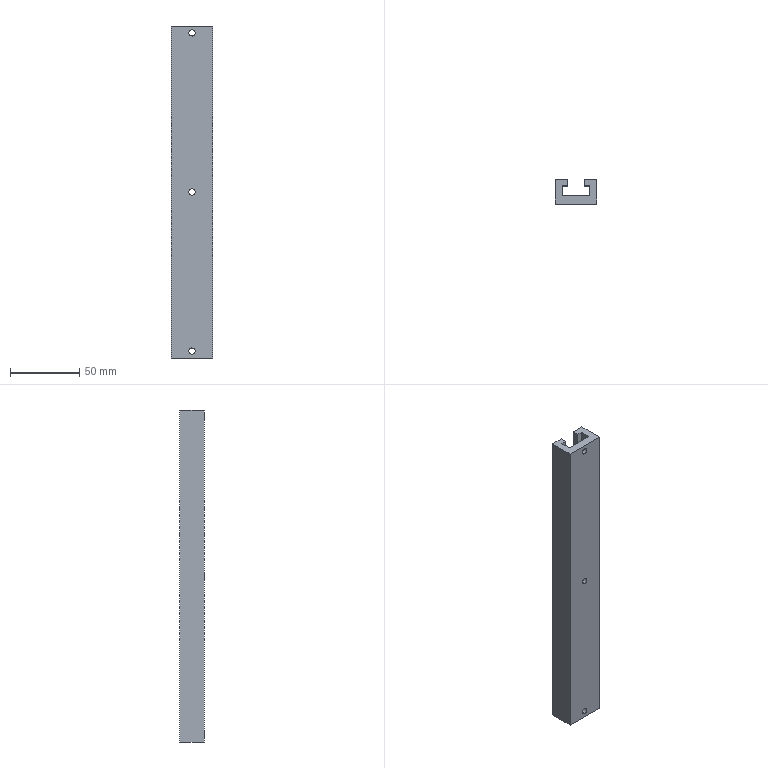Part | NX | features BREP 1 | 1 solid | 26 faces | box 30 x 18 x 240 mm | volume 80211 mm3 | plane 14 | cone 6 | cylinder 6 | commonest cylinder face diameters 4.5 x6
STEP:
#1=CARTESIAN_POINT('',(0.,6.,110.5));
#2=VERTEX_POINT('',#1);
#3=CARTESIAN_POINT('',(0.,3.75,112.75));
#4=VERTEX_POINT('',#3);
#5=CARTESIAN_POINT('',(0.,6.,110.5));
#6=DIRECTION('',(0.,0.7071,-0.7071));
#7=VECTOR('',#6,1000.);
#8=LINE('',#5,#7);
#9=EDGE_CURVE('',#2,#4,#8,.F.);
#10=ORIENTED_EDGE('',*,*,#9,.T.);
#11=CARTESIAN_POINT('',(0.,3.75,117.25));
#12=VERTEX_POINT('',#11);
#13=CARTESIAN_POINT('',(0.,3.75,115.));
#14=DIRECTION('',(0.,1.,0.));
#15=DIRECTION('',(0.,0.,1.));
#16=AXIS2_PLACEMENT_3D('',#13,#14,#15);
#17=CIRCLE('',#16,2.25);
#18=EDGE_CURVE('',#12,#4,#17,.T.);
#19=ORIENTED_EDGE('',*,*,#18,.F.);
#20=CARTESIAN_POINT('',(0.,6.,119.5));
#21=VERTEX_POINT('',#20);
#22=CARTESIAN_POINT('',(0.,6.,119.5));
#23=DIRECTION('',(0.,0.7071,0.7071));
#24=VECTOR('',#23,1000.);
#25=LINE('',#22,#24);
#26=EDGE_CURVE('',#21,#12,#25,.F.);
#27=ORIENTED_EDGE('',*,*,#26,.F.);
#28=CARTESIAN_POINT('',(0.,6.,115.));
#29=DIRECTION('',(0.,1.,0.));
#30=DIRECTION('',(0.,0.,1.));
#31=AXIS2_PLACEMENT_3D('',#28,#29,#30);
#32=CIRCLE('',#31,4.5);
#33=EDGE_CURVE('',#21,#2,#32,.T.);
#34=ORIENTED_EDGE('',*,*,#33,.T.);
#35=EDGE_LOOP('',(#10,#19,#27,#34));
#36=FACE_BOUND('',#35,.T.);
#37=CARTESIAN_POINT('',(0.,6.,115.));
#38=DIRECTION('',(0.,1.,0.));
#39=DIRECTION('',(0.,0.,1.));
#40=AXIS2_PLACEMENT_3D('',#37,#38,#39);
#41=CONICAL_SURFACE('',#40,4.5,0.7854);
#42=ADVANCED_FACE('',(#36),#41,.F.);
#43=CARTESIAN_POINT('',(0.,0.,112.75));
#44=VERTEX_POINT('',#43);
#45=CARTESIAN_POINT('',(0.,6.,112.75));
#46=DIRECTION('',(0.,1.,0.));
#47=VECTOR('',#46,1000.);
#48=LINE('',#45,#47);
#49=EDGE_CURVE('',#4,#44,#48,.F.);
#50=ORIENTED_EDGE('',*,*,#49,.T.);
#51=CARTESIAN_POINT('',(0.,0.,117.25));
#52=VERTEX_POINT('',#51);
#53=CARTESIAN_POINT('',(0.,0.,115.));
#54=DIRECTION('',(0.,1.,0.));
#55=DIRECTION('',(0.,0.,1.));
#56=AXIS2_PLACEMENT_3D('',#53,#54,#55);
#57=CIRCLE('',#56,2.25);
#58=EDGE_CURVE('',#52,#44,#57,.T.);
#59=ORIENTED_EDGE('',*,*,#58,.F.);
#60=CARTESIAN_POINT('',(0.,6.,117.25));
#61=DIRECTION('',(0.,1.,0.));
#62=VECTOR('',#61,1000.);
#63=LINE('',#60,#62);
#64=EDGE_CURVE('',#12,#52,#63,.F.);
#65=ORIENTED_EDGE('',*,*,#64,.F.);
#66=ORIENTED_EDGE('',*,*,#18,.T.);
#67=EDGE_LOOP('',(#50,#59,#65,#66));
#68=FACE_BOUND('',#67,.T.);
#69=CARTESIAN_POINT('',(0.,6.,115.));
#70=DIRECTION('',(0.,1.,0.));
#71=DIRECTION('',(0.,0.,1.));
#72=AXIS2_PLACEMENT_3D('',#69,#70,#71);
#73=CYLINDRICAL_SURFACE('',#72,2.25);
#74=ADVANCED_FACE('',(#68),#73,.F.);
#75=CARTESIAN_POINT('',(0.,6.,-4.5));
#76=VERTEX_POINT('',#75);
#77=CARTESIAN_POINT('',(0.,3.75,-2.25));
#78=VERTEX_POINT('',#77);
#79=CARTESIAN_POINT('',(0.,6.,-4.5));
#80=DIRECTION('',(0.,0.7071,-0.7071));
#81=VECTOR('',#80,1000.);
#82=LINE('',#79,#81);
#83=EDGE_CURVE('',#76,#78,#82,.F.);
#84=ORIENTED_EDGE('',*,*,#83,.T.);
#85=CARTESIAN_POINT('',(0.,3.75,2.25));
#86=VERTEX_POINT('',#85);
#87=CARTESIAN_POINT('',(0.,3.75,0.));
#88=DIRECTION('',(0.,1.,0.));
#89=DIRECTION('',(0.,0.,1.));
#90=AXIS2_PLACEMENT_3D('',#87,#88,#89);
#91=CIRCLE('',#90,2.25);
#92=EDGE_CURVE('',#86,#78,#91,.T.);
#93=ORIENTED_EDGE('',*,*,#92,.F.);
#94=CARTESIAN_POINT('',(0.,6.,4.5));
#95=VERTEX_POINT('',#94);
#96=CARTESIAN_POINT('',(0.,6.,4.5));
#97=DIRECTION('',(0.,0.7071,0.7071));
#98=VECTOR('',#97,1000.);
#99=LINE('',#96,#98);
#100=EDGE_CURVE('',#95,#86,#99,.F.);
#101=ORIENTED_EDGE('',*,*,#100,.F.);
#102=CARTESIAN_POINT('',(0.,6.,0.));
#103=DIRECTION('',(0.,1.,0.));
#104=DIRECTION('',(0.,0.,1.));
#105=AXIS2_PLACEMENT_3D('',#102,#103,#104);
#106=CIRCLE('',#105,4.5);
#107=EDGE_CURVE('',#95,#76,#106,.T.);
#108=ORIENTED_EDGE('',*,*,#107,.T.);
#109=EDGE_LOOP('',(#84,#93,#101,#108));
#110=FACE_BOUND('',#109,.T.);
#111=CARTESIAN_POINT('',(0.,6.,0.));
#112=DIRECTION('',(0.,1.,0.));
#113=DIRECTION('',(0.,0.,1.));
#114=AXIS2_PLACEMENT_3D('',#111,#112,#113);
#115=CONICAL_SURFACE('',#114,4.5,0.7854);
#116=ADVANCED_FACE('',(#110),#115,.F.);
#117=CARTESIAN_POINT('',(0.,0.,-2.25));
#118=VERTEX_POINT('',#117);
#119=CARTESIAN_POINT('',(0.,6.,-2.25));
#120=DIRECTION('',(0.,1.,0.));
#121=VECTOR('',#120,1000.);
#122=LINE('',#119,#121);
#123=EDGE_CURVE('',#78,#118,#122,.F.);
#124=ORIENTED_EDGE('',*,*,#123,.T.);
#125=CARTESIAN_POINT('',(0.,0.,2.25));
#126=VERTEX_POINT('',#125);
#127=CARTESIAN_POINT('',(0.,0.,0.));
#128=DIRECTION('',(0.,1.,0.));
#129=DIRECTION('',(0.,0.,1.));
#130=AXIS2_PLACEMENT_3D('',#127,#128,#129);
#131=CIRCLE('',#130,2.25);
#132=EDGE_CURVE('',#126,#118,#131,.T.);
#133=ORIENTED_EDGE('',*,*,#132,.F.);
#134=CARTESIAN_POINT('',(0.,6.,2.25));
#135=DIRECTION('',(0.,1.,0.));
#136=VECTOR('',#135,1000.);
#137=LINE('',#134,#136);
#138=EDGE_CURVE('',#86,#126,#137,.F.);
#139=ORIENTED_EDGE('',*,*,#138,.F.);
#140=ORIENTED_EDGE('',*,*,#92,.T.);
#141=EDGE_LOOP('',(#124,#133,#139,#140));
#142=FACE_BOUND('',#141,.T.);
#143=CARTESIAN_POINT('',(0.,6.,0.));
#144=DIRECTION('',(0.,1.,0.));
#145=DIRECTION('',(0.,0.,1.));
#146=AXIS2_PLACEMENT_3D('',#143,#144,#145);
#147=CYLINDRICAL_SURFACE('',#146,2.25);
#148=ADVANCED_FACE('',(#142),#147,.F.);
#149=CARTESIAN_POINT('',(0.,6.,-119.5));
#150=VERTEX_POINT('',#149);
#151=CARTESIAN_POINT('',(0.,3.75,-117.25));
#152=VERTEX_POINT('',#151);
#153=CARTESIAN_POINT('',(0.,6.,-119.5));
#154=DIRECTION('',(0.,0.7071,-0.7071));
#155=VECTOR('',#154,1000.);
#156=LINE('',#153,#155);
#157=EDGE_CURVE('',#150,#152,#156,.F.);
#158=ORIENTED_EDGE('',*,*,#157,.T.);
#159=CARTESIAN_POINT('',(0.,3.75,-112.75));
#160=VERTEX_POINT('',#159);
#161=CARTESIAN_POINT('',(0.,3.75,-115.));
#162=DIRECTION('',(0.,1.,0.));
#163=DIRECTION('',(0.,0.,1.));
#164=AXIS2_PLACEMENT_3D('',#161,#162,#163);
#165=CIRCLE('',#164,2.25);
#166=EDGE_CURVE('',#160,#152,#165,.T.);
#167=ORIENTED_EDGE('',*,*,#166,.F.);
#168=CARTESIAN_POINT('',(0.,6.,-110.5));
#169=VERTEX_POINT('',#168);
#170=CARTESIAN_POINT('',(0.,6.,-110.5));
#171=DIRECTION('',(0.,0.7071,0.7071));
#172=VECTOR('',#171,1000.);
#173=LINE('',#170,#172);
#174=EDGE_CURVE('',#169,#160,#173,.F.);
#175=ORIENTED_EDGE('',*,*,#174,.F.);
#176=CARTESIAN_POINT('',(0.,6.,-115.));
#177=DIRECTION('',(0.,1.,0.));
#178=DIRECTION('',(0.,0.,1.));
#179=AXIS2_PLACEMENT_3D('',#176,#177,#178);
#180=CIRCLE('',#179,4.5);
#181=EDGE_CURVE('',#169,#150,#180,.T.);
#182=ORIENTED_EDGE('',*,*,#181,.T.);
#183=EDGE_LOOP('',(#158,#167,#175,#182));
#184=FACE_BOUND('',#183,.T.);
#185=CARTESIAN_POINT('',(0.,6.,-115.));
#186=DIRECTION('',(0.,1.,0.));
#187=DIRECTION('',(0.,0.,1.));
#188=AXIS2_PLACEMENT_3D('',#185,#186,#187);
#189=CONICAL_SURFACE('',#188,4.5,0.7854);
#190=ADVANCED_FACE('',(#184),#189,.F.);
#191=CARTESIAN_POINT('',(0.,0.,-117.25));
#192=VERTEX_POINT('',#191);
#193=CARTESIAN_POINT('',(0.,6.,-117.25));
#194=DIRECTION('',(0.,1.,0.));
#195=VECTOR('',#194,1000.);
#196=LINE('',#193,#195);
#197=EDGE_CURVE('',#152,#192,#196,.F.);
#198=ORIENTED_EDGE('',*,*,#197,.T.);
#199=CARTESIAN_POINT('',(0.,0.,-112.75));
#200=VERTEX_POINT('',#199);
#201=CARTESIAN_POINT('',(0.,0.,-115.));
#202=DIRECTION('',(0.,1.,0.));
#203=DIRECTION('',(0.,0.,1.));
#204=AXIS2_PLACEMENT_3D('',#201,#202,#203);
#205=CIRCLE('',#204,2.25);
#206=EDGE_CURVE('',#200,#192,#205,.T.);
#207=ORIENTED_EDGE('',*,*,#206,.F.);
#208=CARTESIAN_POINT('',(0.,6.,-112.75));
#209=DIRECTION('',(0.,1.,0.));
#210=VECTOR('',#209,1000.);
#211=LINE('',#208,#210);
#212=EDGE_CURVE('',#160,#200,#211,.F.);
#213=ORIENTED_EDGE('',*,*,#212,.F.);
#214=ORIENTED_EDGE('',*,*,#166,.T.);
#215=EDGE_LOOP('',(#198,#207,#213,#214));
#216=FACE_BOUND('',#215,.T.);
#217=CARTESIAN_POINT('',(0.,6.,-115.));
#218=DIRECTION('',(0.,1.,0.));
#219=DIRECTION('',(0.,0.,1.));
#220=AXIS2_PLACEMENT_3D('',#217,#218,#219);
#221=CYLINDRICAL_SURFACE('',#220,2.25);
#222=ADVANCED_FACE('',(#216),#221,.F.);
#223=CARTESIAN_POINT('',(10.,13.5,-120.));
#224=VERTEX_POINT('',#223);
#225=CARTESIAN_POINT('',(10.,6.,-120.));
#226=VERTEX_POINT('',#225);
#227=CARTESIAN_POINT('',(10.,13.5,-120.));
#228=DIRECTION('',(0.,-1.,0.));
#229=VECTOR('',#228,1000.);
#230=LINE('',#227,#229);
#231=EDGE_CURVE('',#224,#226,#230,.T.);
#232=ORIENTED_EDGE('',*,*,#231,.F.);
#233=CARTESIAN_POINT('',(6.,13.5,-120.));
#234=VERTEX_POINT('',#233);
#235=CARTESIAN_POINT('',(6.,13.5,-120.));
#236=DIRECTION('',(1.,0.,0.));
#237=VECTOR('',#236,1000.);
#238=LINE('',#235,#237);
#239=EDGE_CURVE('',#234,#224,#238,.T.);
#240=ORIENTED_EDGE('',*,*,#239,.F.);
#241=CARTESIAN_POINT('',(6.,18.,-120.));
#242=VERTEX_POINT('',#241);
#243=CARTESIAN_POINT('',(6.,18.,-120.));
#244=DIRECTION('',(0.,-1.,0.));
#245=VECTOR('',#244,1000.);
#246=LINE('',#243,#245);
#247=EDGE_CURVE('',#242,#234,#246,.T.);
#248=ORIENTED_EDGE('',*,*,#247,.F.);
#249=CARTESIAN_POINT('',(15.,18.,-120.));
#250=VERTEX_POINT('',#249);
#251=CARTESIAN_POINT('',(15.,18.,-120.));
#252=DIRECTION('',(-1.,0.,0.));
#253=VECTOR('',#252,1000.);
#254=LINE('',#251,#253);
#255=EDGE_CURVE('',#250,#242,#254,.T.);
#256=ORIENTED_EDGE('',*,*,#255,.F.);
#257=CARTESIAN_POINT('',(15.,0.,-120.));
#258=VERTEX_POINT('',#257);
#259=CARTESIAN_POINT('',(15.,0.,-120.));
#260=DIRECTION('',(0.,1.,0.));
#261=VECTOR('',#260,1000.);
#262=LINE('',#259,#261);
#263=EDGE_CURVE('',#258,#250,#262,.T.);
#264=ORIENTED_EDGE('',*,*,#263,.F.);
#265=CARTESIAN_POINT('',(-15.,0.,-120.));
#266=VERTEX_POINT('',#265);
#267=CARTESIAN_POINT('',(15.,0.,-120.));
#268=DIRECTION('',(1.,0.,0.));
#269=VECTOR('',#268,1000.);
#270=LINE('',#267,#269);
#271=EDGE_CURVE('',#266,#258,#270,.T.);
#272=ORIENTED_EDGE('',*,*,#271,.F.);
#273=CARTESIAN_POINT('',(-15.,18.,-120.));
#274=VERTEX_POINT('',#273);
#275=CARTESIAN_POINT('',(-15.,0.,-120.));
#276=DIRECTION('',(0.,-1.,0.));
#277=VECTOR('',#276,1000.);
#278=LINE('',#275,#277);
#279=EDGE_CURVE('',#274,#266,#278,.T.);
#280=ORIENTED_EDGE('',*,*,#279,.F.);
#281=CARTESIAN_POINT('',(-6.,18.,-120.));
#282=VERTEX_POINT('',#281);
#283=CARTESIAN_POINT('',(-15.,18.,-120.));
#284=DIRECTION('',(-1.,0.,0.));
#285=VECTOR('',#284,1000.);
#286=LINE('',#283,#285);
#287=EDGE_CURVE('',#282,#274,#286,.T.);
#288=ORIENTED_EDGE('',*,*,#287,.F.);
#289=CARTESIAN_POINT('',(-6.,13.5,-120.));
#290=VERTEX_POINT('',#289);
#291=CARTESIAN_POINT('',(-6.,18.,-120.));
#292=DIRECTION('',(0.,1.,0.));
#293=VECTOR('',#292,1000.);
#294=LINE('',#291,#293);
#295=EDGE_CURVE('',#290,#282,#294,.T.);
#296=ORIENTED_EDGE('',*,*,#295,.F.);
#297=CARTESIAN_POINT('',(-10.,13.5,-120.));
#298=VERTEX_POINT('',#297);
#299=CARTESIAN_POINT('',(-6.,13.5,-120.));
#300=DIRECTION('',(1.,0.,0.));
#301=VECTOR('',#300,1000.);
#302=LINE('',#299,#301);
#303=EDGE_CURVE('',#298,#290,#302,.T.);
#304=ORIENTED_EDGE('',*,*,#303,.F.);
#305=CARTESIAN_POINT('',(-10.,6.,-120.));
#306=VERTEX_POINT('',#305);
#307=CARTESIAN_POINT('',(-10.,13.5,-120.));
#308=DIRECTION('',(0.,1.,0.));
#309=VECTOR('',#308,1000.);
#310=LINE('',#307,#309);
#311=EDGE_CURVE('',#306,#298,#310,.T.);
#312=ORIENTED_EDGE('',*,*,#311,.F.);
#313=CARTESIAN_POINT('',(-10.,6.,-120.));
#314=DIRECTION('',(-1.,0.,0.));
#315=VECTOR('',#314,1000.);
#316=LINE('',#313,#315);
#317=EDGE_CURVE('',#226,#306,#316,.T.);
#318=ORIENTED_EDGE('',*,*,#317,.F.);
#319=EDGE_LOOP('',(#232,#240,#248,#256,#264,#272,#280,#288,#296,#304,#312,#318));
#320=FACE_BOUND('',#319,.T.);
#321=CARTESIAN_POINT('',(0.,0.,-120.));
#322=DIRECTION('',(0.,0.,1.));
#323=DIRECTION('',(1.,0.,0.));
#324=AXIS2_PLACEMENT_3D('',#321,#322,#323);
#325=PLANE('',#324);
#326=ADVANCED_FACE('',(#320),#325,.F.);
#327=CARTESIAN_POINT('',(10.,13.5,120.));
#328=VERTEX_POINT('',#327);
#329=CARTESIAN_POINT('',(10.,6.,120.));
#330=VERTEX_POINT('',#329);
#331=CARTESIAN_POINT('',(10.,13.5,120.));
#332=DIRECTION('',(0.,-1.,0.));
#333=VECTOR('',#332,1000.);
#334=LINE('',#331,#333);
#335=EDGE_CURVE('',#328,#330,#334,.T.);
#336=ORIENTED_EDGE('',*,*,#335,.T.);
#337=CARTESIAN_POINT('',(-10.,6.,120.));
#338=VERTEX_POINT('',#337);
#339=CARTESIAN_POINT('',(-10.,6.,120.));
#340=DIRECTION('',(-1.,0.,0.));
#341=VECTOR('',#340,1000.);
#342=LINE('',#339,#341);
#343=EDGE_CURVE('',#330,#338,#342,.T.);
#344=ORIENTED_EDGE('',*,*,#343,.T.);
#345=CARTESIAN_POINT('',(-10.,13.5,120.));
#346=VERTEX_POINT('',#345);
#347=CARTESIAN_POINT('',(-10.,13.5,120.));
#348=DIRECTION('',(0.,1.,0.));
#349=VECTOR('',#348,1000.);
#350=LINE('',#347,#349);
#351=EDGE_CURVE('',#338,#346,#350,.T.);
#352=ORIENTED_EDGE('',*,*,#351,.T.);
#353=CARTESIAN_POINT('',(-6.,13.5,120.));
#354=VERTEX_POINT('',#353);
#355=CARTESIAN_POINT('',(-6.,13.5,120.));
#356=DIRECTION('',(1.,0.,0.));
#357=VECTOR('',#356,1000.);
#358=LINE('',#355,#357);
#359=EDGE_CURVE('',#346,#354,#358,.T.);
#360=ORIENTED_EDGE('',*,*,#359,.T.);
#361=CARTESIAN_POINT('',(-6.,18.,120.));
#362=VERTEX_POINT('',#361);
#363=CARTESIAN_POINT('',(-6.,18.,120.));
#364=DIRECTION('',(0.,1.,0.));
#365=VECTOR('',#364,1000.);
#366=LINE('',#363,#365);
#367=EDGE_CURVE('',#354,#362,#366,.T.);
#368=ORIENTED_EDGE('',*,*,#367,.T.);
#369=CARTESIAN_POINT('',(-15.,18.,120.));
#370=VERTEX_POINT('',#369);
#371=CARTESIAN_POINT('',(-15.,18.,120.));
#372=DIRECTION('',(-1.,0.,0.));
#373=VECTOR('',#372,1000.);
#374=LINE('',#371,#373);
#375=EDGE_CURVE('',#362,#370,#374,.T.);
#376=ORIENTED_EDGE('',*,*,#375,.T.);
#377=CARTESIAN_POINT('',(-15.,0.,120.));
#378=VERTEX_POINT('',#377);
#379=CARTESIAN_POINT('',(-15.,0.,120.));
#380=DIRECTION('',(0.,-1.,0.));
#381=VECTOR('',#380,1000.);
#382=LINE('',#379,#381);
#383=EDGE_CURVE('',#370,#378,#382,.T.);
#384=ORIENTED_EDGE('',*,*,#383,.T.);
#385=CARTESIAN_POINT('',(15.,0.,120.));
#386=VERTEX_POINT('',#385);
#387=CARTESIAN_POINT('',(15.,0.,120.));
#388=DIRECTION('',(1.,0.,0.));
#389=VECTOR('',#388,1000.);
#390=LINE('',#387,#389);
#391=EDGE_CURVE('',#378,#386,#390,.T.);
#392=ORIENTED_EDGE('',*,*,#391,.T.);
#393=CARTESIAN_POINT('',(15.,18.,120.));
#394=VERTEX_POINT('',#393);
#395=CARTESIAN_POINT('',(15.,0.,120.));
#396=DIRECTION('',(0.,1.,0.));
#397=VECTOR('',#396,1000.);
#398=LINE('',#395,#397);
#399=EDGE_CURVE('',#386,#394,#398,.T.);
#400=ORIENTED_EDGE('',*,*,#399,.T.);
#401=CARTESIAN_POINT('',(6.,18.,120.));
#402=VERTEX_POINT('',#401);
#403=CARTESIAN_POINT('',(15.,18.,120.));
#404=DIRECTION('',(-1.,0.,0.));
#405=VECTOR('',#404,1000.);
#406=LINE('',#403,#405);
#407=EDGE_CURVE('',#394,#402,#406,.T.);
#408=ORIENTED_EDGE('',*,*,#407,.T.);
#409=CARTESIAN_POINT('',(6.,13.5,120.));
#410=VERTEX_POINT('',#409);
#411=CARTESIAN_POINT('',(6.,18.,120.));
#412=DIRECTION('',(0.,-1.,0.));
#413=VECTOR('',#412,1000.);
#414=LINE('',#411,#413);
#415=EDGE_CURVE('',#402,#410,#414,.T.);
#416=ORIENTED_EDGE('',*,*,#415,.T.);
#417=CARTESIAN_POINT('',(6.,13.5,120.));
#418=DIRECTION('',(1.,0.,0.));
#419=VECTOR('',#418,1000.);
#420=LINE('',#417,#419);
#421=EDGE_CURVE('',#410,#328,#420,.T.);
#422=ORIENTED_EDGE('',*,*,#421,.T.);
#423=EDGE_LOOP('',(#336,#344,#352,#360,#368,#376,#384,#392,#400,#408,#416,#422));
#424=FACE_BOUND('',#423,.T.);
#425=CARTESIAN_POINT('',(0.,0.,120.));
#426=DIRECTION('',(0.,0.,1.));
#427=DIRECTION('',(1.,0.,0.));
#428=AXIS2_PLACEMENT_3D('',#425,#426,#427);
#429=PLANE('',#428);
#430=ADVANCED_FACE('',(#424),#429,.T.);
#431=ORIENTED_EDGE('',*,*,#239,.T.);
#432=CARTESIAN_POINT('',(10.,13.5,120.));
#433=DIRECTION('',(0.,0.,-1.));
#434=VECTOR('',#433,1000.);
#435=LINE('',#432,#434);
#436=EDGE_CURVE('',#328,#224,#435,.T.);
#437=ORIENTED_EDGE('',*,*,#436,.F.);
#438=ORIENTED_EDGE('',*,*,#421,.F.);
#439=CARTESIAN_POINT('',(6.,13.5,120.));
#440=DIRECTION('',(0.,0.,-1.));
#441=VECTOR('',#440,1000.);
#442=LINE('',#439,#441);
#443=EDGE_CURVE('',#410,#234,#442,.T.);
#444=ORIENTED_EDGE('',*,*,#443,.T.);
#445=EDGE_LOOP('',(#431,#437,#438,#444));
#446=FACE_BOUND('',#445,.T.);
#447=CARTESIAN_POINT('',(6.,13.5,120.));
#448=DIRECTION('',(0.,1.,0.));
#449=DIRECTION('',(-1.,0.,0.));
#450=AXIS2_PLACEMENT_3D('',#447,#448,#449);
#451=PLANE('',#450);
#452=ADVANCED_FACE('',(#446),#451,.F.);
#453=ORIENTED_EDGE('',*,*,#247,.T.);
#454=ORIENTED_EDGE('',*,*,#443,.F.);
#455=ORIENTED_EDGE('',*,*,#415,.F.);
#456=CARTESIAN_POINT('',(6.,18.,120.));
#457=DIRECTION('',(0.,0.,-1.));
#458=VECTOR('',#457,1000.);
#459=LINE('',#456,#458);
#460=EDGE_CURVE('',#402,#242,#459,.T.);
#461=ORIENTED_EDGE('',*,*,#460,.T.);
#462=EDGE_LOOP('',(#453,#454,#455,#461));
#463=FACE_BOUND('',#462,.T.);
#464=CARTESIAN_POINT('',(6.,18.,120.));
#465=DIRECTION('',(1.,0.,0.));
#466=DIRECTION('',(0.,1.,0.));
#467=AXIS2_PLACEMENT_3D('',#464,#465,#466);
#468=PLANE('',#467);
#469=ADVANCED_FACE('',(#463),#468,.F.);
#470=ORIENTED_EDGE('',*,*,#255,.T.);
#471=ORIENTED_EDGE('',*,*,#460,.F.);
#472=ORIENTED_EDGE('',*,*,#407,.F.);
#473=CARTESIAN_POINT('',(15.,18.,120.));
#474=DIRECTION('',(0.,0.,-1.));
#475=VECTOR('',#474,1000.);
#476=LINE('',#473,#475);
#477=EDGE_CURVE('',#394,#250,#476,.T.);
#478=ORIENTED_EDGE('',*,*,#477,.T.);
#479=EDGE_LOOP('',(#470,#471,#472,#478));
#480=FACE_BOUND('',#479,.T.);
#481=CARTESIAN_POINT('',(15.,18.,120.));
#482=DIRECTION('',(0.,-1.,0.));
#483=DIRECTION('',(0.,0.,-1.));
#484=AXIS2_PLACEMENT_3D('',#481,#482,#483);
#485=PLANE('',#484);
#486=ADVANCED_FACE('',(#480),#485,.F.);
#487=ORIENTED_EDGE('',*,*,#263,.T.);
#488=ORIENTED_EDGE('',*,*,#477,.F.);
#489=ORIENTED_EDGE('',*,*,#399,.F.);
#490=CARTESIAN_POINT('',(15.,0.,120.));
#491=DIRECTION('',(0.,0.,-1.));
#492=VECTOR('',#491,1000.);
#493=LINE('',#490,#492);
#494=EDGE_CURVE('',#386,#258,#493,.T.);
#495=ORIENTED_EDGE('',*,*,#494,.T.);
#496=EDGE_LOOP('',(#487,#488,#489,#495));
#497=FACE_BOUND('',#496,.T.);
#498=CARTESIAN_POINT('',(15.,0.,120.));
#499=DIRECTION('',(-1.,0.,0.));
#500=DIRECTION('',(0.,0.,1.));
#501=AXIS2_PLACEMENT_3D('',#498,#499,#500);
#502=PLANE('',#501);
#503=ADVANCED_FACE('',(#497),#502,.F.);
#504=ORIENTED_EDGE('',*,*,#271,.T.);
#505=ORIENTED_EDGE('',*,*,#494,.F.);
#506=ORIENTED_EDGE('',*,*,#391,.F.);
#507=CARTESIAN_POINT('',(-15.,0.,120.));
#508=DIRECTION('',(0.,0.,-1.));
#509=VECTOR('',#508,1000.);
#510=LINE('',#507,#509);
#511=EDGE_CURVE('',#378,#266,#510,.T.);
#512=ORIENTED_EDGE('',*,*,#511,.T.);
#513=EDGE_LOOP('',(#504,#505,#506,#512));
#514=FACE_BOUND('',#513,.T.);
#515=ORIENTED_EDGE('',*,*,#206,.T.);
#516=CARTESIAN_POINT('',(0.,0.,-115.));
#517=DIRECTION('',(0.,1.,0.));
#518=DIRECTION('',(0.,0.,1.));
#519=AXIS2_PLACEMENT_3D('',#516,#517,#518);
#520=CIRCLE('',#519,2.25);
#521=EDGE_CURVE('',#192,#200,#520,.T.);
#522=ORIENTED_EDGE('',*,*,#521,.T.);
#523=EDGE_LOOP('',(#515,#522));
#524=FACE_BOUND('',#523,.T.);
#525=ORIENTED_EDGE('',*,*,#132,.T.);
#526=CARTESIAN_POINT('',(0.,0.,0.));
#527=DIRECTION('',(0.,1.,0.));
#528=DIRECTION('',(0.,0.,1.));
#529=AXIS2_PLACEMENT_3D('',#526,#527,#528);
#530=CIRCLE('',#529,2.25);
#531=EDGE_CURVE('',#118,#126,#530,.T.);
#532=ORIENTED_EDGE('',*,*,#531,.T.);
#533=EDGE_LOOP('',(#525,#532));
#534=FACE_BOUND('',#533,.T.);
#535=ORIENTED_EDGE('',*,*,#58,.T.);
#536=CARTESIAN_POINT('',(0.,0.,115.));
#537=DIRECTION('',(0.,1.,0.));
#538=DIRECTION('',(0.,0.,1.));
#539=AXIS2_PLACEMENT_3D('',#536,#537,#538);
#540=CIRCLE('',#539,2.25);
#541=EDGE_CURVE('',#44,#52,#540,.T.);
#542=ORIENTED_EDGE('',*,*,#541,.T.);
#543=EDGE_LOOP('',(#535,#542));
#544=FACE_BOUND('',#543,.T.);
#545=CARTESIAN_POINT('',(15.,0.,120.));
#546=DIRECTION('',(0.,1.,0.));
#547=DIRECTION('',(0.,0.,1.));
#548=AXIS2_PLACEMENT_3D('',#545,#546,#547);
#549=PLANE('',#548);
#550=ADVANCED_FACE('',(#514,#524,#534,#544),#549,.F.);
#551=ORIENTED_EDGE('',*,*,#279,.T.);
#552=ORIENTED_EDGE('',*,*,#511,.F.);
#553=ORIENTED_EDGE('',*,*,#383,.F.);
#554=CARTESIAN_POINT('',(-15.,18.,120.));
#555=DIRECTION('',(0.,0.,-1.));
#556=VECTOR('',#555,1000.);
#557=LINE('',#554,#556);
#558=EDGE_CURVE('',#370,#274,#557,.T.);
#559=ORIENTED_EDGE('',*,*,#558,.T.);
#560=EDGE_LOOP('',(#551,#552,#553,#559));
#561=FACE_BOUND('',#560,.T.);
#562=CARTESIAN_POINT('',(-15.,0.,120.));
#563=DIRECTION('',(1.,0.,0.));
#564=DIRECTION('',(0.,0.,-1.));
#565=AXIS2_PLACEMENT_3D('',#562,#563,#564);
#566=PLANE('',#565);
#567=ADVANCED_FACE('',(#561),#566,.F.);
#568=ORIENTED_EDGE('',*,*,#287,.T.);
#569=ORIENTED_EDGE('',*,*,#558,.F.);
#570=ORIENTED_EDGE('',*,*,#375,.F.);
#571=CARTESIAN_POINT('',(-6.,18.,120.));
#572=DIRECTION('',(0.,0.,-1.));
#573=VECTOR('',#572,1000.);
#574=LINE('',#571,#573);
#575=EDGE_CURVE('',#362,#282,#574,.T.);
#576=ORIENTED_EDGE('',*,*,#575,.T.);
#577=EDGE_LOOP('',(#568,#569,#570,#576));
#578=FACE_BOUND('',#577,.T.);
#579=CARTESIAN_POINT('',(-15.,18.,120.));
#580=DIRECTION('',(0.,-1.,0.));
#581=DIRECTION('',(0.,0.,-1.));
#582=AXIS2_PLACEMENT_3D('',#579,#580,#581);
#583=PLANE('',#582);
#584=ADVANCED_FACE('',(#578),#583,.F.);
#585=ORIENTED_EDGE('',*,*,#295,.T.);
#586=ORIENTED_EDGE('',*,*,#575,.F.);
#587=ORIENTED_EDGE('',*,*,#367,.F.);
#588=CARTESIAN_POINT('',(-6.,13.5,120.));
#589=DIRECTION('',(0.,0.,-1.));
#590=VECTOR('',#589,1000.);
#591=LINE('',#588,#590);
#592=EDGE_CURVE('',#354,#290,#591,.T.);
#593=ORIENTED_EDGE('',*,*,#592,.T.);
#594=EDGE_LOOP('',(#585,#586,#587,#593));
#595=FACE_BOUND('',#594,.T.);
#596=CARTESIAN_POINT('',(-6.,18.,120.));
#597=DIRECTION('',(-1.,0.,0.));
#598=DIRECTION('',(0.,-1.,0.));
#599=AXIS2_PLACEMENT_3D('',#596,#597,#598);
#600=PLANE('',#599);
#601=ADVANCED_FACE('',(#595),#600,.F.);
#602=ORIENTED_EDGE('',*,*,#303,.T.);
#603=ORIENTED_EDGE('',*,*,#592,.F.);
#604=ORIENTED_EDGE('',*,*,#359,.F.);
#605=CARTESIAN_POINT('',(-10.,13.5,120.));
#606=DIRECTION('',(0.,0.,-1.));
#607=VECTOR('',#606,1000.);
#608=LINE('',#605,#607);
#609=EDGE_CURVE('',#346,#298,#608,.T.);
#610=ORIENTED_EDGE('',*,*,#609,.T.);
#611=EDGE_LOOP('',(#602,#603,#604,#610));
#612=FACE_BOUND('',#611,.T.);
#613=CARTESIAN_POINT('',(-6.,13.5,120.));
#614=DIRECTION('',(0.,1.,0.));
#615=DIRECTION('',(-1.,0.,0.));
#616=AXIS2_PLACEMENT_3D('',#613,#614,#615);
#617=PLANE('',#616);
#618=ADVANCED_FACE('',(#612),#617,.F.);
#619=ORIENTED_EDGE('',*,*,#311,.T.);
#620=ORIENTED_EDGE('',*,*,#609,.F.);
#621=ORIENTED_EDGE('',*,*,#351,.F.);
#622=CARTESIAN_POINT('',(-10.,6.,120.));
#623=DIRECTION('',(0.,0.,-1.));
#624=VECTOR('',#623,1000.);
#625=LINE('',#622,#624);
#626=EDGE_CURVE('',#338,#306,#625,.T.);
#627=ORIENTED_EDGE('',*,*,#626,.T.);
#628=EDGE_LOOP('',(#619,#620,#621,#627));
#629=FACE_BOUND('',#628,.T.);
#630=CARTESIAN_POINT('',(-10.,13.5,120.));
#631=DIRECTION('',(-1.,0.,0.));
#632=DIRECTION('',(0.,-1.,0.));
#633=AXIS2_PLACEMENT_3D('',#630,#631,#632);
#634=PLANE('',#633);
#635=ADVANCED_FACE('',(#629),#634,.F.);
#636=ORIENTED_EDGE('',*,*,#317,.T.);
#637=ORIENTED_EDGE('',*,*,#626,.F.);
#638=ORIENTED_EDGE('',*,*,#343,.F.);
#639=CARTESIAN_POINT('',(10.,6.,120.));
#640=DIRECTION('',(0.,0.,-1.));
#641=VECTOR('',#640,1000.);
#642=LINE('',#639,#641);
#643=EDGE_CURVE('',#330,#226,#642,.T.);
#644=ORIENTED_EDGE('',*,*,#643,.T.);
#645=EDGE_LOOP('',(#636,#637,#638,#644));
#646=FACE_BOUND('',#645,.T.);
#647=ORIENTED_EDGE('',*,*,#181,.F.);
#648=CARTESIAN_POINT('',(0.,6.,-115.));
#649=DIRECTION('',(0.,1.,0.));
#650=DIRECTION('',(0.,0.,1.));
#651=AXIS2_PLACEMENT_3D('',#648,#649,#650);
#652=CIRCLE('',#651,4.5);
#653=EDGE_CURVE('',#150,#169,#652,.T.);
#654=ORIENTED_EDGE('',*,*,#653,.F.);
#655=EDGE_LOOP('',(#647,#654));
#656=FACE_BOUND('',#655,.T.);
#657=ORIENTED_EDGE('',*,*,#107,.F.);
#658=CARTESIAN_POINT('',(0.,6.,0.));
#659=DIRECTION('',(0.,1.,0.));
#660=DIRECTION('',(0.,0.,1.));
#661=AXIS2_PLACEMENT_3D('',#658,#659,#660);
#662=CIRCLE('',#661,4.5);
#663=EDGE_CURVE('',#76,#95,#662,.T.);
#664=ORIENTED_EDGE('',*,*,#663,.F.);
#665=EDGE_LOOP('',(#657,#664));
#666=FACE_BOUND('',#665,.T.);
#667=ORIENTED_EDGE('',*,*,#33,.F.);
#668=CARTESIAN_POINT('',(0.,6.,115.));
#669=DIRECTION('',(0.,1.,0.));
#670=DIRECTION('',(0.,0.,1.));
#671=AXIS2_PLACEMENT_3D('',#668,#669,#670);
#672=CIRCLE('',#671,4.5);
#673=EDGE_CURVE('',#2,#21,#672,.T.);
#674=ORIENTED_EDGE('',*,*,#673,.F.);
#675=EDGE_LOOP('',(#667,#674));
#676=FACE_BOUND('',#675,.T.);
#677=CARTESIAN_POINT('',(-10.,6.,120.));
#678=DIRECTION('',(0.,-1.,0.));
#679=DIRECTION('',(0.,0.,-1.));
#680=AXIS2_PLACEMENT_3D('',#677,#678,#679);
#681=PLANE('',#680);
#682=ADVANCED_FACE('',(#646,#656,#666,#676),#681,.F.);
#683=ORIENTED_EDGE('',*,*,#231,.T.);
#684=ORIENTED_EDGE('',*,*,#643,.F.);
#685=ORIENTED_EDGE('',*,*,#335,.F.);
#686=ORIENTED_EDGE('',*,*,#436,.T.);
#687=EDGE_LOOP('',(#683,#684,#685,#686));
#688=FACE_BOUND('',#687,.T.);
#689=CARTESIAN_POINT('',(10.,13.5,120.));
#690=DIRECTION('',(1.,0.,0.));
#691=DIRECTION('',(0.,1.,0.));
#692=AXIS2_PLACEMENT_3D('',#689,#690,#691);
#693=PLANE('',#692);
#694=ADVANCED_FACE('',(#688),#693,.F.);
#695=ORIENTED_EDGE('',*,*,#521,.F.);
#696=ORIENTED_EDGE('',*,*,#197,.F.);
#697=CARTESIAN_POINT('',(0.,3.75,-115.));
#698=DIRECTION('',(0.,1.,0.));
#699=DIRECTION('',(0.,0.,1.));
#700=AXIS2_PLACEMENT_3D('',#697,#698,#699);
#701=CIRCLE('',#700,2.25);
#702=EDGE_CURVE('',#152,#160,#701,.T.);
#703=ORIENTED_EDGE('',*,*,#702,.T.);
#704=ORIENTED_EDGE('',*,*,#212,.T.);
#705=EDGE_LOOP('',(#695,#696,#703,#704));
#706=FACE_BOUND('',#705,.T.);
#707=CARTESIAN_POINT('',(0.,6.,-115.));
#708=DIRECTION('',(0.,1.,0.));
#709=DIRECTION('',(0.,0.,1.));
#710=AXIS2_PLACEMENT_3D('',#707,#708,#709);
#711=CYLINDRICAL_SURFACE('',#710,2.25);
#712=ADVANCED_FACE('',(#706),#711,.F.);
#713=ORIENTED_EDGE('',*,*,#702,.F.);
#714=ORIENTED_EDGE('',*,*,#157,.F.);
#715=ORIENTED_EDGE('',*,*,#653,.T.);
#716=ORIENTED_EDGE('',*,*,#174,.T.);
#717=EDGE_LOOP('',(#713,#714,#715,#716));
#718=FACE_BOUND('',#717,.T.);
#719=CARTESIAN_POINT('',(0.,6.,-115.));
#720=DIRECTION('',(0.,1.,0.));
#721=DIRECTION('',(0.,0.,1.));
#722=AXIS2_PLACEMENT_3D('',#719,#720,#721);
#723=CONICAL_SURFACE('',#722,4.5,0.7854);
#724=ADVANCED_FACE('',(#718),#723,.F.);
#725=ORIENTED_EDGE('',*,*,#531,.F.);
#726=ORIENTED_EDGE('',*,*,#123,.F.);
#727=CARTESIAN_POINT('',(0.,3.75,0.));
#728=DIRECTION('',(0.,1.,0.));
#729=DIRECTION('',(0.,0.,1.));
#730=AXIS2_PLACEMENT_3D('',#727,#728,#729);
#731=CIRCLE('',#730,2.25);
#732=EDGE_CURVE('',#78,#86,#731,.T.);
#733=ORIENTED_EDGE('',*,*,#732,.T.);
#734=ORIENTED_EDGE('',*,*,#138,.T.);
#735=EDGE_LOOP('',(#725,#726,#733,#734));
#736=FACE_BOUND('',#735,.T.);
#737=CARTESIAN_POINT('',(0.,6.,0.));
#738=DIRECTION('',(0.,1.,0.));
#739=DIRECTION('',(0.,0.,1.));
#740=AXIS2_PLACEMENT_3D('',#737,#738,#739);
#741=CYLINDRICAL_SURFACE('',#740,2.25);
#742=ADVANCED_FACE('',(#736),#741,.F.);
#743=ORIENTED_EDGE('',*,*,#732,.F.);
#744=ORIENTED_EDGE('',*,*,#83,.F.);
#745=ORIENTED_EDGE('',*,*,#663,.T.);
#746=ORIENTED_EDGE('',*,*,#100,.T.);
#747=EDGE_LOOP('',(#743,#744,#745,#746));
#748=FACE_BOUND('',#747,.T.);
#749=CARTESIAN_POINT('',(0.,6.,0.));
#750=DIRECTION('',(0.,1.,0.));
#751=DIRECTION('',(0.,0.,1.));
#752=AXIS2_PLACEMENT_3D('',#749,#750,#751);
#753=CONICAL_SURFACE('',#752,4.5,0.7854);
#754=ADVANCED_FACE('',(#748),#753,.F.);
#755=ORIENTED_EDGE('',*,*,#541,.F.);
#756=ORIENTED_EDGE('',*,*,#49,.F.);
#757=CARTESIAN_POINT('',(0.,3.75,115.));
#758=DIRECTION('',(0.,1.,0.));
#759=DIRECTION('',(0.,0.,1.));
#760=AXIS2_PLACEMENT_3D('',#757,#758,#759);
#761=CIRCLE('',#760,2.25);
#762=EDGE_CURVE('',#4,#12,#761,.T.);
#763=ORIENTED_EDGE('',*,*,#762,.T.);
#764=ORIENTED_EDGE('',*,*,#64,.T.);
#765=EDGE_LOOP('',(#755,#756,#763,#764));
#766=FACE_BOUND('',#765,.T.);
#767=CARTESIAN_POINT('',(0.,6.,115.));
#768=DIRECTION('',(0.,1.,0.));
#769=DIRECTION('',(0.,0.,1.));
#770=AXIS2_PLACEMENT_3D('',#767,#768,#769);
#771=CYLINDRICAL_SURFACE('',#770,2.25);
#772=ADVANCED_FACE('',(#766),#771,.F.);
#773=ORIENTED_EDGE('',*,*,#762,.F.);
#774=ORIENTED_EDGE('',*,*,#9,.F.);
#775=ORIENTED_EDGE('',*,*,#673,.T.);
#776=ORIENTED_EDGE('',*,*,#26,.T.);
#777=EDGE_LOOP('',(#773,#774,#775,#776));
#778=FACE_BOUND('',#777,.T.);
#779=CARTESIAN_POINT('',(0.,6.,115.));
#780=DIRECTION('',(0.,1.,0.));
#781=DIRECTION('',(0.,0.,1.));
#782=AXIS2_PLACEMENT_3D('',#779,#780,#781);
#783=CONICAL_SURFACE('',#782,4.5,0.7854);
#784=ADVANCED_FACE('',(#778),#783,.F.);
#785=CLOSED_SHELL('',(#42,#74,#116,#148,#190,#222,#326,#430,#452,#469,#486,#503,#550,#567,#584,#601,#618,#635,#682,#694,#712,#724,#742,#754,#772,#784));
#786=MANIFOLD_SOLID_BREP('',#785);
#787=(LENGTH_UNIT()NAMED_UNIT(*)SI_UNIT(.MILLI.,.METRE.));
#788=UNCERTAINTY_MEASURE_WITH_UNIT(LENGTH_MEASURE(0.00001),#787,'','');
#789=(NAMED_UNIT(*)PLANE_ANGLE_UNIT()SI_UNIT($,.RADIAN.));
#790=(NAMED_UNIT(*)SI_UNIT($,.STERADIAN.)SOLID_ANGLE_UNIT());
#791=(GEOMETRIC_REPRESENTATION_CONTEXT(3)GLOBAL_UNCERTAINTY_ASSIGNED_CONTEXT((#788))GLOBAL_UNIT_ASSIGNED_CONTEXT((#787,#789,#790))REPRESENTATION_CONTEXT('',''));
#792=ADVANCED_BREP_SHAPE_REPRESENTATION('',(#786),#791);